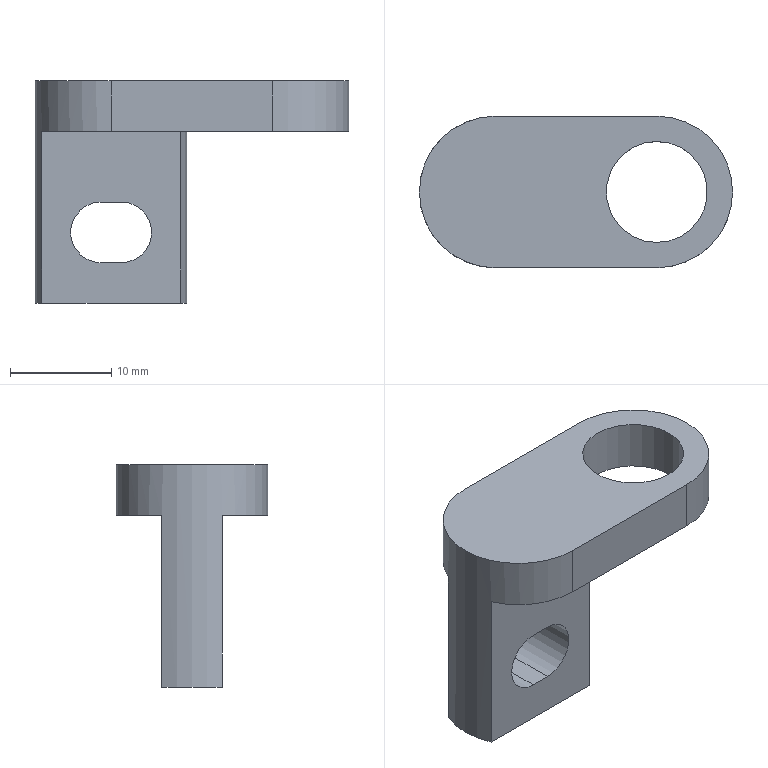Part | NX | features BREP 1, DATUM_CSYS 1 | 1 solid | 15 faces | box 31 x 15 x 22 mm | volume 2937 mm3 | plane 9 | cylinder 6 | commonest cylinder face diameters 15 x3 6 x2 10 x1
STEP:
#1=CARTESIAN_POINT('',(16.,-7.5,0.));
#2=VERTEX_POINT('',#1);
#3=CARTESIAN_POINT('',(16.,7.5,0.));
#4=VERTEX_POINT('',#3);
#5=CARTESIAN_POINT('',(16.,0.,0.));
#6=DIRECTION('',(0.,0.,1.));
#7=DIRECTION('',(0.,-1.,0.));
#8=AXIS2_PLACEMENT_3D('',#5,#6,#7);
#9=CIRCLE('',#8,7.5);
#10=EDGE_CURVE('',#2,#4,#9,.T.);
#11=ORIENTED_EDGE('',*,*,#10,.F.);
#12=CARTESIAN_POINT('',(0.,-7.5,0.));
#13=VERTEX_POINT('',#12);
#14=CARTESIAN_POINT('',(0.,-7.5,0.));
#15=DIRECTION('',(1.,0.,0.));
#16=VECTOR('',#15,1000.);
#17=LINE('',#14,#16);
#18=EDGE_CURVE('',#13,#2,#17,.T.);
#19=ORIENTED_EDGE('',*,*,#18,.F.);
#20=CARTESIAN_POINT('',(-6.874,-3.,0.));
#21=VERTEX_POINT('',#20);
#22=CARTESIAN_POINT('',(0.,0.,0.));
#23=DIRECTION('',(0.,0.,-1.));
#24=DIRECTION('',(0.,-1.,0.));
#25=AXIS2_PLACEMENT_3D('',#22,#23,#24);
#26=CIRCLE('',#25,7.5);
#27=EDGE_CURVE('',#13,#21,#26,.T.);
#28=ORIENTED_EDGE('',*,*,#27,.T.);
#29=CARTESIAN_POINT('',(6.874,-3.,0.));
#30=VERTEX_POINT('',#29);
#31=CARTESIAN_POINT('',(-6.874,-3.,0.));
#32=DIRECTION('',(1.,0.,0.));
#33=VECTOR('',#32,1000.);
#34=LINE('',#31,#33);
#35=EDGE_CURVE('',#21,#30,#34,.T.);
#36=ORIENTED_EDGE('',*,*,#35,.T.);
#37=CARTESIAN_POINT('',(6.874,3.,0.));
#38=VERTEX_POINT('',#37);
#39=CARTESIAN_POINT('',(0.,0.,0.));
#40=DIRECTION('',(0.,0.,-1.));
#41=DIRECTION('',(0.9165,0.4,0.));
#42=AXIS2_PLACEMENT_3D('',#39,#40,#41);
#43=CIRCLE('',#42,7.5);
#44=EDGE_CURVE('',#38,#30,#43,.T.);
#45=ORIENTED_EDGE('',*,*,#44,.F.);
#46=CARTESIAN_POINT('',(-6.874,3.,0.));
#47=VERTEX_POINT('',#46);
#48=CARTESIAN_POINT('',(6.874,3.,0.));
#49=DIRECTION('',(-1.,0.,0.));
#50=VECTOR('',#49,1000.);
#51=LINE('',#48,#50);
#52=EDGE_CURVE('',#38,#47,#51,.T.);
#53=ORIENTED_EDGE('',*,*,#52,.T.);
#54=CARTESIAN_POINT('',(0.,7.5,0.));
#55=VERTEX_POINT('',#54);
#56=CARTESIAN_POINT('',(0.,0.,0.));
#57=DIRECTION('',(0.,0.,-1.));
#58=DIRECTION('',(-0.9165,0.4,0.));
#59=AXIS2_PLACEMENT_3D('',#56,#57,#58);
#60=CIRCLE('',#59,7.5);
#61=EDGE_CURVE('',#47,#55,#60,.T.);
#62=ORIENTED_EDGE('',*,*,#61,.T.);
#63=CARTESIAN_POINT('',(16.,7.5,0.));
#64=DIRECTION('',(-1.,0.,0.));
#65=VECTOR('',#64,1000.);
#66=LINE('',#63,#65);
#67=EDGE_CURVE('',#4,#55,#66,.T.);
#68=ORIENTED_EDGE('',*,*,#67,.F.);
#69=EDGE_LOOP('',(#11,#19,#28,#36,#45,#53,#62,#68));
#70=FACE_BOUND('',#69,.T.);
#71=CARTESIAN_POINT('',(16.,-5.,0.));
#72=VERTEX_POINT('',#71);
#73=CARTESIAN_POINT('',(16.,0.,0.));
#74=DIRECTION('',(0.,0.,-1.));
#75=DIRECTION('',(0.,-1.,0.));
#76=AXIS2_PLACEMENT_3D('',#73,#74,#75);
#77=CIRCLE('',#76,5.);
#78=EDGE_CURVE('',#72,#72,#77,.T.);
#79=ORIENTED_EDGE('',*,*,#78,.F.);
#80=EDGE_LOOP('',(#79));
#81=FACE_BOUND('',#80,.T.);
#82=CARTESIAN_POINT('',(0.,-4.382,0.));
#83=DIRECTION('',(0.,0.,1.));
#84=DIRECTION('',(-1.,0.,0.));
#85=AXIS2_PLACEMENT_3D('',#82,#83,#84);
#86=PLANE('',#85);
#87=ADVANCED_FACE('',(#70,#81),#86,.F.);
#88=ORIENTED_EDGE('',*,*,#18,.T.);
#89=CARTESIAN_POINT('',(16.,-7.5,5.));
#90=VERTEX_POINT('',#89);
#91=CARTESIAN_POINT('',(16.,-7.5,0.));
#92=DIRECTION('',(0.,0.,1.));
#93=VECTOR('',#92,1000.);
#94=LINE('',#91,#93);
#95=EDGE_CURVE('',#2,#90,#94,.T.);
#96=ORIENTED_EDGE('',*,*,#95,.T.);
#97=CARTESIAN_POINT('',(0.,-7.5,5.));
#98=VERTEX_POINT('',#97);
#99=CARTESIAN_POINT('',(0.,-7.5,5.));
#100=DIRECTION('',(1.,0.,0.));
#101=VECTOR('',#100,1000.);
#102=LINE('',#99,#101);
#103=EDGE_CURVE('',#98,#90,#102,.T.);
#104=ORIENTED_EDGE('',*,*,#103,.F.);
#105=CARTESIAN_POINT('',(0.,-7.5,0.));
#106=DIRECTION('',(0.,0.,1.));
#107=VECTOR('',#106,1000.);
#108=LINE('',#105,#107);
#109=EDGE_CURVE('',#13,#98,#108,.T.);
#110=ORIENTED_EDGE('',*,*,#109,.F.);
#111=EDGE_LOOP('',(#88,#96,#104,#110));
#112=FACE_BOUND('',#111,.T.);
#113=CARTESIAN_POINT('',(8.,-7.5,2.5));
#114=DIRECTION('',(0.,-1.,0.));
#115=DIRECTION('',(-1.,0.,0.));
#116=AXIS2_PLACEMENT_3D('',#113,#114,#115);
#117=PLANE('',#116);
#118=ADVANCED_FACE('',(#112),#117,.T.);
#119=ORIENTED_EDGE('',*,*,#10,.T.);
#120=CARTESIAN_POINT('',(16.,7.5,5.));
#121=VERTEX_POINT('',#120);
#122=CARTESIAN_POINT('',(16.,7.5,0.));
#123=DIRECTION('',(0.,0.,1.));
#124=VECTOR('',#123,1000.);
#125=LINE('',#122,#124);
#126=EDGE_CURVE('',#4,#121,#125,.T.);
#127=ORIENTED_EDGE('',*,*,#126,.T.);
#128=CARTESIAN_POINT('',(16.,0.,5.));
#129=DIRECTION('',(0.,0.,1.));
#130=DIRECTION('',(0.,-1.,0.));
#131=AXIS2_PLACEMENT_3D('',#128,#129,#130);
#132=CIRCLE('',#131,7.5);
#133=EDGE_CURVE('',#90,#121,#132,.T.);
#134=ORIENTED_EDGE('',*,*,#133,.F.);
#135=ORIENTED_EDGE('',*,*,#95,.F.);
#136=EDGE_LOOP('',(#119,#127,#134,#135));
#137=FACE_BOUND('',#136,.T.);
#138=CARTESIAN_POINT('',(16.,0.,0.));
#139=DIRECTION('',(0.,0.,1.));
#140=DIRECTION('',(0.,1.,0.));
#141=AXIS2_PLACEMENT_3D('',#138,#139,#140);
#142=CYLINDRICAL_SURFACE('',#141,7.5);
#143=ADVANCED_FACE('',(#137),#142,.T.);
#144=ORIENTED_EDGE('',*,*,#67,.T.);
#145=CARTESIAN_POINT('',(0.,7.5,5.));
#146=VERTEX_POINT('',#145);
#147=CARTESIAN_POINT('',(0.,7.5,0.));
#148=DIRECTION('',(0.,0.,1.));
#149=VECTOR('',#148,1000.);
#150=LINE('',#147,#149);
#151=EDGE_CURVE('',#55,#146,#150,.T.);
#152=ORIENTED_EDGE('',*,*,#151,.T.);
#153=CARTESIAN_POINT('',(16.,7.5,5.));
#154=DIRECTION('',(-1.,0.,0.));
#155=VECTOR('',#154,1000.);
#156=LINE('',#153,#155);
#157=EDGE_CURVE('',#121,#146,#156,.T.);
#158=ORIENTED_EDGE('',*,*,#157,.F.);
#159=ORIENTED_EDGE('',*,*,#126,.F.);
#160=EDGE_LOOP('',(#144,#152,#158,#159));
#161=FACE_BOUND('',#160,.T.);
#162=CARTESIAN_POINT('',(8.,7.5,2.5));
#163=DIRECTION('',(0.,1.,0.));
#164=DIRECTION('',(1.,0.,0.));
#165=AXIS2_PLACEMENT_3D('',#162,#163,#164);
#166=PLANE('',#165);
#167=ADVANCED_FACE('',(#161),#166,.T.);
#168=CARTESIAN_POINT('',(16.,-5.,5.));
#169=VERTEX_POINT('',#168);
#170=CARTESIAN_POINT('',(16.,-5.,5.));
#171=DIRECTION('',(0.,0.,-1.));
#172=VECTOR('',#171,1000.);
#173=LINE('',#170,#172);
#174=EDGE_CURVE('',#169,#72,#173,.T.);
#175=ORIENTED_EDGE('',*,*,#174,.T.);
#176=ORIENTED_EDGE('',*,*,#78,.T.);
#177=ORIENTED_EDGE('',*,*,#174,.F.);
#178=CARTESIAN_POINT('',(16.,0.,5.));
#179=DIRECTION('',(0.,0.,-1.));
#180=DIRECTION('',(0.,-1.,0.));
#181=AXIS2_PLACEMENT_3D('',#178,#179,#180);
#182=CIRCLE('',#181,5.);
#183=EDGE_CURVE('',#169,#169,#182,.T.);
#184=ORIENTED_EDGE('',*,*,#183,.F.);
#185=EDGE_LOOP('',(#175,#176,#177,#184));
#186=FACE_BOUND('',#185,.T.);
#187=CARTESIAN_POINT('',(16.,0.,5.));
#188=DIRECTION('',(0.,0.,-1.));
#189=DIRECTION('',(0.,1.,0.));
#190=AXIS2_PLACEMENT_3D('',#187,#188,#189);
#191=CYLINDRICAL_SURFACE('',#190,5.);
#192=ADVANCED_FACE('',(#186),#191,.F.);
#193=ORIENTED_EDGE('',*,*,#103,.T.);
#194=ORIENTED_EDGE('',*,*,#133,.T.);
#195=ORIENTED_EDGE('',*,*,#157,.T.);
#196=CARTESIAN_POINT('',(0.,0.,5.));
#197=DIRECTION('',(0.,0.,1.));
#198=DIRECTION('',(0.,1.,0.));
#199=AXIS2_PLACEMENT_3D('',#196,#197,#198);
#200=CIRCLE('',#199,7.5);
#201=EDGE_CURVE('',#146,#98,#200,.T.);
#202=ORIENTED_EDGE('',*,*,#201,.T.);
#203=EDGE_LOOP('',(#193,#194,#195,#202));
#204=FACE_BOUND('',#203,.T.);
#205=ORIENTED_EDGE('',*,*,#183,.T.);
#206=EDGE_LOOP('',(#205));
#207=FACE_BOUND('',#206,.T.);
#208=CARTESIAN_POINT('',(6.9,6.9,5.));
#209=DIRECTION('',(0.,0.,1.));
#210=DIRECTION('',(-1.,0.,0.));
#211=AXIS2_PLACEMENT_3D('',#208,#209,#210);
#212=PLANE('',#211);
#213=ADVANCED_FACE('',(#204,#207),#212,.T.);
#214=CARTESIAN_POINT('',(6.874,-3.,-17.));
#215=VERTEX_POINT('',#214);
#216=CARTESIAN_POINT('',(6.874,3.,-17.));
#217=VERTEX_POINT('',#216);
#218=CARTESIAN_POINT('',(0.,0.,-17.));
#219=DIRECTION('',(0.,0.,1.));
#220=DIRECTION('',(0.9165,-0.4,0.));
#221=AXIS2_PLACEMENT_3D('',#218,#219,#220);
#222=CIRCLE('',#221,7.5);
#223=EDGE_CURVE('',#215,#217,#222,.T.);
#224=ORIENTED_EDGE('',*,*,#223,.F.);
#225=CARTESIAN_POINT('',(-6.874,-3.,-17.));
#226=VERTEX_POINT('',#225);
#227=CARTESIAN_POINT('',(-6.874,-3.,-17.));
#228=DIRECTION('',(1.,0.,0.));
#229=VECTOR('',#228,1000.);
#230=LINE('',#227,#229);
#231=EDGE_CURVE('',#226,#215,#230,.T.);
#232=ORIENTED_EDGE('',*,*,#231,.F.);
#233=CARTESIAN_POINT('',(-6.874,3.,-17.));
#234=VERTEX_POINT('',#233);
#235=CARTESIAN_POINT('',(0.,0.,-17.));
#236=DIRECTION('',(0.,0.,1.));
#237=DIRECTION('',(-0.9165,0.4,0.));
#238=AXIS2_PLACEMENT_3D('',#235,#236,#237);
#239=CIRCLE('',#238,7.5);
#240=EDGE_CURVE('',#234,#226,#239,.T.);
#241=ORIENTED_EDGE('',*,*,#240,.F.);
#242=CARTESIAN_POINT('',(6.874,3.,-17.));
#243=DIRECTION('',(-1.,0.,0.));
#244=VECTOR('',#243,1000.);
#245=LINE('',#242,#244);
#246=EDGE_CURVE('',#217,#234,#245,.T.);
#247=ORIENTED_EDGE('',*,*,#246,.F.);
#248=EDGE_LOOP('',(#224,#232,#241,#247));
#249=FACE_BOUND('',#248,.T.);
#250=CARTESIAN_POINT('',(0.,0.,-17.));
#251=DIRECTION('',(0.,0.,-1.));
#252=DIRECTION('',(0.,-1.,0.));
#253=AXIS2_PLACEMENT_3D('',#250,#251,#252);
#254=PLANE('',#253);
#255=ADVANCED_FACE('',(#249),#254,.T.);
#256=ORIENTED_EDGE('',*,*,#109,.T.);
#257=ORIENTED_EDGE('',*,*,#201,.F.);
#258=ORIENTED_EDGE('',*,*,#151,.F.);
#259=ORIENTED_EDGE('',*,*,#61,.F.);
#260=CARTESIAN_POINT('',(-6.874,3.,-17.));
#261=DIRECTION('',(0.,0.,1.));
#262=VECTOR('',#261,1000.);
#263=LINE('',#260,#262);
#264=EDGE_CURVE('',#234,#47,#263,.T.);
#265=ORIENTED_EDGE('',*,*,#264,.F.);
#266=ORIENTED_EDGE('',*,*,#240,.T.);
#267=CARTESIAN_POINT('',(-6.874,-3.,0.));
#268=DIRECTION('',(0.,0.,-1.));
#269=VECTOR('',#268,1000.);
#270=LINE('',#267,#269);
#271=EDGE_CURVE('',#21,#226,#270,.T.);
#272=ORIENTED_EDGE('',*,*,#271,.F.);
#273=ORIENTED_EDGE('',*,*,#27,.F.);
#274=EDGE_LOOP('',(#256,#257,#258,#259,#265,#266,#272,#273));
#275=FACE_BOUND('',#274,.T.);
#276=CARTESIAN_POINT('',(0.,0.,5.));
#277=DIRECTION('',(0.,0.,-1.));
#278=DIRECTION('',(0.,1.,0.));
#279=AXIS2_PLACEMENT_3D('',#276,#277,#278);
#280=CYLINDRICAL_SURFACE('',#279,7.5);
#281=ADVANCED_FACE('',(#275),#280,.T.);
#282=ORIENTED_EDGE('',*,*,#223,.T.);
#283=CARTESIAN_POINT('',(6.874,3.,0.));
#284=DIRECTION('',(0.,0.,-1.));
#285=VECTOR('',#284,1000.);
#286=LINE('',#283,#285);
#287=EDGE_CURVE('',#38,#217,#286,.T.);
#288=ORIENTED_EDGE('',*,*,#287,.F.);
#289=ORIENTED_EDGE('',*,*,#44,.T.);
#290=CARTESIAN_POINT('',(6.874,-3.,-17.));
#291=DIRECTION('',(0.,0.,1.));
#292=VECTOR('',#291,1000.);
#293=LINE('',#290,#292);
#294=EDGE_CURVE('',#215,#30,#293,.T.);
#295=ORIENTED_EDGE('',*,*,#294,.F.);
#296=EDGE_LOOP('',(#282,#288,#289,#295));
#297=FACE_BOUND('',#296,.T.);
#298=CARTESIAN_POINT('',(0.,0.,5.));
#299=DIRECTION('',(0.,0.,-1.));
#300=DIRECTION('',(0.,1.,0.));
#301=AXIS2_PLACEMENT_3D('',#298,#299,#300);
#302=CYLINDRICAL_SURFACE('',#301,7.5);
#303=ADVANCED_FACE('',(#297),#302,.T.);
#304=ORIENTED_EDGE('',*,*,#246,.T.);
#305=ORIENTED_EDGE('',*,*,#264,.T.);
#306=ORIENTED_EDGE('',*,*,#52,.F.);
#307=ORIENTED_EDGE('',*,*,#287,.T.);
#308=EDGE_LOOP('',(#304,#305,#306,#307));
#309=FACE_BOUND('',#308,.T.);
#310=CARTESIAN_POINT('',(1.,3.,-13.));
#311=VERTEX_POINT('',#310);
#312=CARTESIAN_POINT('',(-1.,3.,-13.));
#313=VERTEX_POINT('',#312);
#314=CARTESIAN_POINT('',(1.,3.,-13.));
#315=DIRECTION('',(-1.,0.,0.));
#316=VECTOR('',#315,1000.);
#317=LINE('',#314,#316);
#318=EDGE_CURVE('',#311,#313,#317,.T.);
#319=ORIENTED_EDGE('',*,*,#318,.F.);
#320=CARTESIAN_POINT('',(1.,3.,-7.));
#321=VERTEX_POINT('',#320);
#322=CARTESIAN_POINT('',(1.,3.,-10.));
#323=DIRECTION('',(0.,1.,0.));
#324=DIRECTION('',(0.,0.,1.));
#325=AXIS2_PLACEMENT_3D('',#322,#323,#324);
#326=CIRCLE('',#325,3.);
#327=EDGE_CURVE('',#321,#311,#326,.T.);
#328=ORIENTED_EDGE('',*,*,#327,.F.);
#329=CARTESIAN_POINT('',(-1.,3.,-7.));
#330=VERTEX_POINT('',#329);
#331=CARTESIAN_POINT('',(-1.,3.,-7.));
#332=DIRECTION('',(1.,0.,0.));
#333=VECTOR('',#332,1000.);
#334=LINE('',#331,#333);
#335=EDGE_CURVE('',#330,#321,#334,.T.);
#336=ORIENTED_EDGE('',*,*,#335,.F.);
#337=CARTESIAN_POINT('',(-1.,3.,-10.));
#338=DIRECTION('',(0.,1.,0.));
#339=DIRECTION('',(0.,0.,-1.));
#340=AXIS2_PLACEMENT_3D('',#337,#338,#339);
#341=CIRCLE('',#340,3.);
#342=EDGE_CURVE('',#313,#330,#341,.T.);
#343=ORIENTED_EDGE('',*,*,#342,.F.);
#344=EDGE_LOOP('',(#319,#328,#336,#343));
#345=FACE_BOUND('',#344,.T.);
#346=CARTESIAN_POINT('',(0.,3.,-8.5));
#347=DIRECTION('',(0.,1.,0.));
#348=DIRECTION('',(1.,0.,0.));
#349=AXIS2_PLACEMENT_3D('',#346,#347,#348);
#350=PLANE('',#349);
#351=ADVANCED_FACE('',(#309,#345),#350,.T.);
#352=ORIENTED_EDGE('',*,*,#231,.T.);
#353=ORIENTED_EDGE('',*,*,#294,.T.);
#354=ORIENTED_EDGE('',*,*,#35,.F.);
#355=ORIENTED_EDGE('',*,*,#271,.T.);
#356=EDGE_LOOP('',(#352,#353,#354,#355));
#357=FACE_BOUND('',#356,.T.);
#358=CARTESIAN_POINT('',(1.,-3.,-7.));
#359=VERTEX_POINT('',#358);
#360=CARTESIAN_POINT('',(-1.,-3.,-7.));
#361=VERTEX_POINT('',#360);
#362=CARTESIAN_POINT('',(1.,-3.,-7.));
#363=DIRECTION('',(-1.,0.,0.));
#364=VECTOR('',#363,1000.);
#365=LINE('',#362,#364);
#366=EDGE_CURVE('',#359,#361,#365,.T.);
#367=ORIENTED_EDGE('',*,*,#366,.F.);
#368=CARTESIAN_POINT('',(1.,-3.,-13.));
#369=VERTEX_POINT('',#368);
#370=CARTESIAN_POINT('',(1.,-3.,-10.));
#371=DIRECTION('',(0.,-1.,0.));
#372=DIRECTION('',(0.,0.,-1.));
#373=AXIS2_PLACEMENT_3D('',#370,#371,#372);
#374=CIRCLE('',#373,3.);
#375=EDGE_CURVE('',#369,#359,#374,.T.);
#376=ORIENTED_EDGE('',*,*,#375,.F.);
#377=CARTESIAN_POINT('',(-1.,-3.,-13.));
#378=VERTEX_POINT('',#377);
#379=CARTESIAN_POINT('',(-1.,-3.,-13.));
#380=DIRECTION('',(1.,0.,0.));
#381=VECTOR('',#380,1000.);
#382=LINE('',#379,#381);
#383=EDGE_CURVE('',#378,#369,#382,.T.);
#384=ORIENTED_EDGE('',*,*,#383,.F.);
#385=CARTESIAN_POINT('',(-1.,-3.,-10.));
#386=DIRECTION('',(0.,-1.,0.));
#387=DIRECTION('',(0.,0.,1.));
#388=AXIS2_PLACEMENT_3D('',#385,#386,#387);
#389=CIRCLE('',#388,3.);
#390=EDGE_CURVE('',#361,#378,#389,.T.);
#391=ORIENTED_EDGE('',*,*,#390,.F.);
#392=EDGE_LOOP('',(#367,#376,#384,#391));
#393=FACE_BOUND('',#392,.T.);
#394=CARTESIAN_POINT('',(0.,-3.,-8.5));
#395=DIRECTION('',(0.,-1.,0.));
#396=DIRECTION('',(-1.,0.,0.));
#397=AXIS2_PLACEMENT_3D('',#394,#395,#396);
#398=PLANE('',#397);
#399=ADVANCED_FACE('',(#357,#393),#398,.T.);
#400=ORIENTED_EDGE('',*,*,#383,.T.);
#401=CARTESIAN_POINT('',(1.,-3.,-13.));
#402=DIRECTION('',(0.,1.,0.));
#403=VECTOR('',#402,1000.);
#404=LINE('',#401,#403);
#405=EDGE_CURVE('',#369,#311,#404,.T.);
#406=ORIENTED_EDGE('',*,*,#405,.T.);
#407=ORIENTED_EDGE('',*,*,#318,.T.);
#408=CARTESIAN_POINT('',(-1.,-3.,-13.));
#409=DIRECTION('',(0.,1.,0.));
#410=VECTOR('',#409,1000.);
#411=LINE('',#408,#410);
#412=EDGE_CURVE('',#378,#313,#411,.T.);
#413=ORIENTED_EDGE('',*,*,#412,.F.);
#414=EDGE_LOOP('',(#400,#406,#407,#413));
#415=FACE_BOUND('',#414,.T.);
#416=CARTESIAN_POINT('',(0.,3.5,-13.));
#417=DIRECTION('',(0.,0.,1.));
#418=DIRECTION('',(-1.,0.,0.));
#419=AXIS2_PLACEMENT_3D('',#416,#417,#418);
#420=PLANE('',#419);
#421=ADVANCED_FACE('',(#415),#420,.T.);
#422=ORIENTED_EDGE('',*,*,#375,.T.);
#423=CARTESIAN_POINT('',(1.,-3.,-7.));
#424=DIRECTION('',(0.,1.,0.));
#425=VECTOR('',#424,1000.);
#426=LINE('',#423,#425);
#427=EDGE_CURVE('',#359,#321,#426,.T.);
#428=ORIENTED_EDGE('',*,*,#427,.T.);
#429=ORIENTED_EDGE('',*,*,#327,.T.);
#430=ORIENTED_EDGE('',*,*,#405,.F.);
#431=EDGE_LOOP('',(#422,#428,#429,#430));
#432=FACE_BOUND('',#431,.T.);
#433=CARTESIAN_POINT('',(1.,-3.,-10.));
#434=DIRECTION('',(0.,1.,0.));
#435=DIRECTION('',(0.,0.,1.));
#436=AXIS2_PLACEMENT_3D('',#433,#434,#435);
#437=CYLINDRICAL_SURFACE('',#436,3.);
#438=ADVANCED_FACE('',(#432),#437,.F.);
#439=ORIENTED_EDGE('',*,*,#366,.T.);
#440=CARTESIAN_POINT('',(-1.,-3.,-7.));
#441=DIRECTION('',(0.,1.,0.));
#442=VECTOR('',#441,1000.);
#443=LINE('',#440,#442);
#444=EDGE_CURVE('',#361,#330,#443,.T.);
#445=ORIENTED_EDGE('',*,*,#444,.T.);
#446=ORIENTED_EDGE('',*,*,#335,.T.);
#447=ORIENTED_EDGE('',*,*,#427,.F.);
#448=EDGE_LOOP('',(#439,#445,#446,#447));
#449=FACE_BOUND('',#448,.T.);
#450=CARTESIAN_POINT('',(0.,3.5,-7.));
#451=DIRECTION('',(0.,0.,-1.));
#452=DIRECTION('',(1.,0.,0.));
#453=AXIS2_PLACEMENT_3D('',#450,#451,#452);
#454=PLANE('',#453);
#455=ADVANCED_FACE('',(#449),#454,.T.);
#456=ORIENTED_EDGE('',*,*,#390,.T.);
#457=ORIENTED_EDGE('',*,*,#412,.T.);
#458=ORIENTED_EDGE('',*,*,#342,.T.);
#459=ORIENTED_EDGE('',*,*,#444,.F.);
#460=EDGE_LOOP('',(#456,#457,#458,#459));
#461=FACE_BOUND('',#460,.T.);
#462=CARTESIAN_POINT('',(-1.,-3.,-10.));
#463=DIRECTION('',(0.,1.,0.));
#464=DIRECTION('',(0.,0.,-1.));
#465=AXIS2_PLACEMENT_3D('',#462,#463,#464);
#466=CYLINDRICAL_SURFACE('',#465,3.);
#467=ADVANCED_FACE('',(#461),#466,.F.);
#468=CLOSED_SHELL('',(#87,#118,#143,#167,#192,#213,#255,#281,#303,#351,#399,#421,#438,#455,#467));
#469=MANIFOLD_SOLID_BREP('',#468);
#470=(LENGTH_UNIT()NAMED_UNIT(*)SI_UNIT(.MILLI.,.METRE.));
#471=UNCERTAINTY_MEASURE_WITH_UNIT(LENGTH_MEASURE(0.00001),#470,'','');
#472=(NAMED_UNIT(*)PLANE_ANGLE_UNIT()SI_UNIT($,.RADIAN.));
#473=(NAMED_UNIT(*)SI_UNIT($,.STERADIAN.)SOLID_ANGLE_UNIT());
#474=(GEOMETRIC_REPRESENTATION_CONTEXT(3)GLOBAL_UNCERTAINTY_ASSIGNED_CONTEXT((#471))GLOBAL_UNIT_ASSIGNED_CONTEXT((#470,#472,#473))REPRESENTATION_CONTEXT('',''));
#475=ADVANCED_BREP_SHAPE_REPRESENTATION('',(#469),#474);